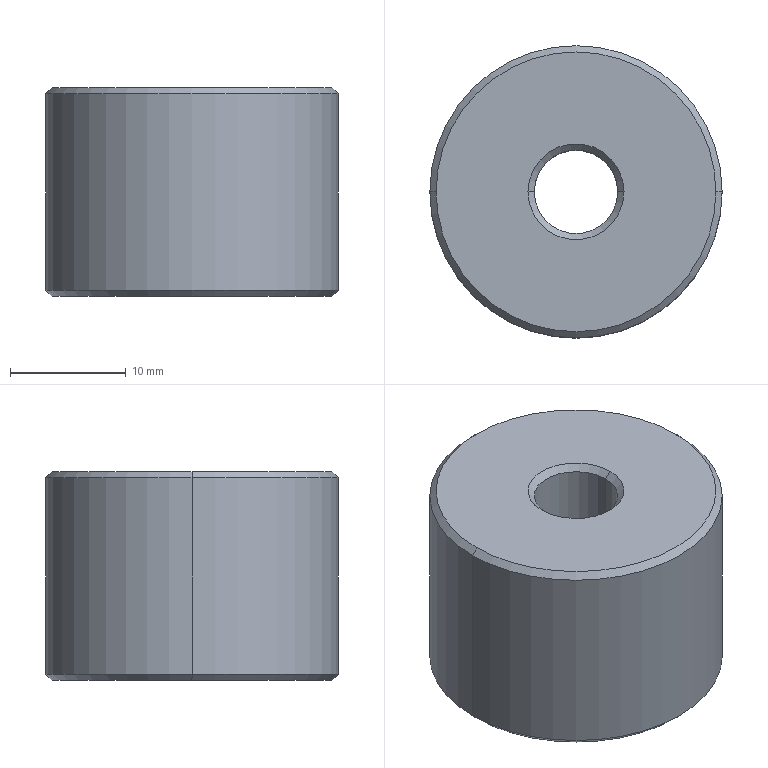Part | SolidWorks | features Chamfer 1, Extrusion 1 | 1 solid | 14 faces | box 25.2 x 25.2 x 18 mm | volume 8215 mm3 | cone 8 | cylinder 4 | plane 2 | commonest cylinder face diameters 7.2 x2 25.2 x2
STEP:
#1=CARTESIAN_POINT('',(12.06,0.,18.));
#2=VERTEX_POINT('',#1);
#3=CARTESIAN_POINT('',(-12.06,0.,18.));
#4=VERTEX_POINT('',#3);
#5=CARTESIAN_POINT('',(0.,0.,18.));
#6=DIRECTION('',(0.,0.,1.));
#7=DIRECTION('',(1.,0.,0.));
#8=AXIS2_PLACEMENT_3D('',#5,#6,#7);
#9=CIRCLE('',#8,12.06);
#10=EDGE_CURVE('',#2,#4,#9,.T.);
#11=ORIENTED_EDGE('',*,*,#10,.F.);
#12=CARTESIAN_POINT('',(12.6,0.,17.46));
#13=VERTEX_POINT('',#12);
#14=CARTESIAN_POINT('',(12.06,0.,18.));
#15=DIRECTION('',(0.7071,0.,-0.7071));
#16=VECTOR('',#15,1000.);
#17=LINE('',#14,#16);
#18=EDGE_CURVE('',#2,#13,#17,.T.);
#19=ORIENTED_EDGE('',*,*,#18,.T.);
#20=CARTESIAN_POINT('',(-12.6,0.,17.46));
#21=VERTEX_POINT('',#20);
#22=CARTESIAN_POINT('',(0.,0.,17.46));
#23=DIRECTION('',(0.,0.,-1.));
#24=DIRECTION('',(1.,0.,0.));
#25=AXIS2_PLACEMENT_3D('',#22,#23,#24);
#26=CIRCLE('',#25,12.6);
#27=EDGE_CURVE('',#21,#13,#26,.T.);
#28=ORIENTED_EDGE('',*,*,#27,.F.);
#29=CARTESIAN_POINT('',(-12.06,0.,18.));
#30=DIRECTION('',(-0.7071,0.,-0.7071));
#31=VECTOR('',#30,1000.);
#32=LINE('',#29,#31);
#33=EDGE_CURVE('',#4,#21,#32,.T.);
#34=ORIENTED_EDGE('',*,*,#33,.F.);
#35=EDGE_LOOP('',(#11,#19,#28,#34));
#36=FACE_OUTER_BOUND('',#35,.T.);
#37=CARTESIAN_POINT('',(0.,0.,18.));
#38=DIRECTION('',(0.,0.,-1.));
#39=DIRECTION('',(-1.,0.,0.));
#40=AXIS2_PLACEMENT_3D('',#37,#38,#39);
#41=CONICAL_SURFACE('',#40,12.06,0.7854);
#42=ADVANCED_FACE('',(#36),#41,.T.);
#43=CARTESIAN_POINT('',(-12.06,0.,0.));
#44=VERTEX_POINT('',#43);
#45=CARTESIAN_POINT('',(12.06,0.,0.));
#46=VERTEX_POINT('',#45);
#47=CARTESIAN_POINT('',(0.,0.,0.));
#48=DIRECTION('',(0.,0.,-1.));
#49=DIRECTION('',(1.,0.,0.));
#50=AXIS2_PLACEMENT_3D('',#47,#48,#49);
#51=CIRCLE('',#50,12.06);
#52=EDGE_CURVE('',#44,#46,#51,.T.);
#53=ORIENTED_EDGE('',*,*,#52,.F.);
#54=CARTESIAN_POINT('',(-12.6,0.,0.54));
#55=VERTEX_POINT('',#54);
#56=CARTESIAN_POINT('',(-12.6,0.,0.54));
#57=DIRECTION('',(-0.7071,0.,0.7071));
#58=VECTOR('',#57,1000.);
#59=LINE('',#56,#58);
#60=EDGE_CURVE('',#44,#55,#59,.T.);
#61=ORIENTED_EDGE('',*,*,#60,.T.);
#62=CARTESIAN_POINT('',(12.6,0.,0.54));
#63=VERTEX_POINT('',#62);
#64=CARTESIAN_POINT('',(0.,0.,0.54));
#65=DIRECTION('',(0.,0.,1.));
#66=DIRECTION('',(1.,0.,0.));
#67=AXIS2_PLACEMENT_3D('',#64,#65,#66);
#68=CIRCLE('',#67,12.6);
#69=EDGE_CURVE('',#63,#55,#68,.T.);
#70=ORIENTED_EDGE('',*,*,#69,.F.);
#71=CARTESIAN_POINT('',(12.6,0.,0.54));
#72=DIRECTION('',(0.7071,0.,0.7071));
#73=VECTOR('',#72,1000.);
#74=LINE('',#71,#73);
#75=EDGE_CURVE('',#46,#63,#74,.T.);
#76=ORIENTED_EDGE('',*,*,#75,.F.);
#77=EDGE_LOOP('',(#53,#61,#70,#76));
#78=FACE_OUTER_BOUND('',#77,.T.);
#79=CARTESIAN_POINT('',(0.,0.,0.54));
#80=DIRECTION('',(0.,0.,1.));
#81=DIRECTION('',(1.,0.,0.));
#82=AXIS2_PLACEMENT_3D('',#79,#80,#81);
#83=CONICAL_SURFACE('',#82,12.6,0.7854);
#84=ADVANCED_FACE('',(#78),#83,.T.);
#85=CARTESIAN_POINT('',(3.6,0.,0.54));
#86=VERTEX_POINT('',#85);
#87=CARTESIAN_POINT('',(-3.6,0.,0.54));
#88=VERTEX_POINT('',#87);
#89=CARTESIAN_POINT('',(0.,0.,0.54));
#90=DIRECTION('',(0.,0.,-1.));
#91=DIRECTION('',(1.,0.,0.));
#92=AXIS2_PLACEMENT_3D('',#89,#90,#91);
#93=CIRCLE('',#92,3.6);
#94=EDGE_CURVE('',#86,#88,#93,.T.);
#95=ORIENTED_EDGE('',*,*,#94,.F.);
#96=CARTESIAN_POINT('',(4.14,0.,0.));
#97=VERTEX_POINT('',#96);
#98=CARTESIAN_POINT('',(4.14,0.,0.));
#99=DIRECTION('',(0.7071,0.,-0.7071));
#100=VECTOR('',#99,1000.);
#101=LINE('',#98,#100);
#102=EDGE_CURVE('',#86,#97,#101,.T.);
#103=ORIENTED_EDGE('',*,*,#102,.T.);
#104=CARTESIAN_POINT('',(-4.14,0.,0.));
#105=VERTEX_POINT('',#104);
#106=CARTESIAN_POINT('',(0.,0.,0.));
#107=DIRECTION('',(0.,0.,1.));
#108=DIRECTION('',(1.,0.,0.));
#109=AXIS2_PLACEMENT_3D('',#106,#107,#108);
#110=CIRCLE('',#109,4.14);
#111=EDGE_CURVE('',#105,#97,#110,.T.);
#112=ORIENTED_EDGE('',*,*,#111,.F.);
#113=CARTESIAN_POINT('',(-4.14,0.,0.));
#114=DIRECTION('',(-0.7071,0.,-0.7071));
#115=VECTOR('',#114,1000.);
#116=LINE('',#113,#115);
#117=EDGE_CURVE('',#88,#105,#116,.T.);
#118=ORIENTED_EDGE('',*,*,#117,.F.);
#119=EDGE_LOOP('',(#95,#103,#112,#118));
#120=FACE_OUTER_BOUND('',#119,.T.);
#121=CARTESIAN_POINT('',(0.,0.,0.));
#122=DIRECTION('',(0.,0.,-1.));
#123=DIRECTION('',(-1.,0.,0.));
#124=AXIS2_PLACEMENT_3D('',#121,#122,#123);
#125=CONICAL_SURFACE('',#124,4.14,0.7854);
#126=ADVANCED_FACE('',(#120),#125,.F.);
#127=CARTESIAN_POINT('',(-3.6,0.,17.46));
#128=VERTEX_POINT('',#127);
#129=CARTESIAN_POINT('',(3.6,0.,17.46));
#130=VERTEX_POINT('',#129);
#131=CARTESIAN_POINT('',(0.,0.,17.46));
#132=DIRECTION('',(0.,0.,1.));
#133=DIRECTION('',(1.,0.,0.));
#134=AXIS2_PLACEMENT_3D('',#131,#132,#133);
#135=CIRCLE('',#134,3.6);
#136=EDGE_CURVE('',#128,#130,#135,.T.);
#137=ORIENTED_EDGE('',*,*,#136,.F.);
#138=CARTESIAN_POINT('',(-4.14,0.,18.));
#139=VERTEX_POINT('',#138);
#140=CARTESIAN_POINT('',(-3.6,0.,17.46));
#141=DIRECTION('',(-0.7071,0.,0.7071));
#142=VECTOR('',#141,1000.);
#143=LINE('',#140,#142);
#144=EDGE_CURVE('',#128,#139,#143,.T.);
#145=ORIENTED_EDGE('',*,*,#144,.T.);
#146=CARTESIAN_POINT('',(4.14,0.,18.));
#147=VERTEX_POINT('',#146);
#148=CARTESIAN_POINT('',(0.,0.,18.));
#149=DIRECTION('',(0.,0.,-1.));
#150=DIRECTION('',(1.,0.,0.));
#151=AXIS2_PLACEMENT_3D('',#148,#149,#150);
#152=CIRCLE('',#151,4.14);
#153=EDGE_CURVE('',#147,#139,#152,.T.);
#154=ORIENTED_EDGE('',*,*,#153,.F.);
#155=CARTESIAN_POINT('',(3.6,0.,17.46));
#156=DIRECTION('',(0.7071,0.,0.7071));
#157=VECTOR('',#156,1000.);
#158=LINE('',#155,#157);
#159=EDGE_CURVE('',#130,#147,#158,.T.);
#160=ORIENTED_EDGE('',*,*,#159,.F.);
#161=EDGE_LOOP('',(#137,#145,#154,#160));
#162=FACE_OUTER_BOUND('',#161,.T.);
#163=CARTESIAN_POINT('',(0.,0.,17.46));
#164=DIRECTION('',(0.,0.,1.));
#165=DIRECTION('',(1.,0.,0.));
#166=AXIS2_PLACEMENT_3D('',#163,#164,#165);
#167=CONICAL_SURFACE('',#166,3.6,0.7854);
#168=ADVANCED_FACE('',(#162),#167,.F.);
#169=ORIENTED_EDGE('',*,*,#136,.T.);
#170=CARTESIAN_POINT('',(3.6,0.,18.));
#171=DIRECTION('',(0.,0.,-1.));
#172=VECTOR('',#171,1000.);
#173=LINE('',#170,#172);
#174=EDGE_CURVE('',#130,#86,#173,.T.);
#175=ORIENTED_EDGE('',*,*,#174,.T.);
#176=ORIENTED_EDGE('',*,*,#94,.T.);
#177=CARTESIAN_POINT('',(-3.6,0.,18.));
#178=DIRECTION('',(0.,0.,-1.));
#179=VECTOR('',#178,1000.);
#180=LINE('',#177,#179);
#181=EDGE_CURVE('',#128,#88,#180,.T.);
#182=ORIENTED_EDGE('',*,*,#181,.F.);
#183=EDGE_LOOP('',(#169,#175,#176,#182));
#184=FACE_OUTER_BOUND('',#183,.T.);
#185=CARTESIAN_POINT('',(0.,0.,18.));
#186=DIRECTION('',(0.,0.,-1.));
#187=DIRECTION('',(-1.,0.,0.));
#188=AXIS2_PLACEMENT_3D('',#185,#186,#187);
#189=CYLINDRICAL_SURFACE('',#188,3.6);
#190=ADVANCED_FACE('',(#184),#189,.F.);
#191=ORIENTED_EDGE('',*,*,#27,.T.);
#192=CARTESIAN_POINT('',(12.6,0.,18.));
#193=DIRECTION('',(0.,0.,-1.));
#194=VECTOR('',#193,1000.);
#195=LINE('',#192,#194);
#196=EDGE_CURVE('',#13,#63,#195,.T.);
#197=ORIENTED_EDGE('',*,*,#196,.T.);
#198=ORIENTED_EDGE('',*,*,#69,.T.);
#199=CARTESIAN_POINT('',(-12.6,0.,18.));
#200=DIRECTION('',(0.,0.,-1.));
#201=VECTOR('',#200,1000.);
#202=LINE('',#199,#201);
#203=EDGE_CURVE('',#21,#55,#202,.T.);
#204=ORIENTED_EDGE('',*,*,#203,.F.);
#205=EDGE_LOOP('',(#191,#197,#198,#204));
#206=FACE_OUTER_BOUND('',#205,.T.);
#207=CARTESIAN_POINT('',(0.,0.,18.));
#208=DIRECTION('',(0.,0.,-1.));
#209=DIRECTION('',(-1.,0.,0.));
#210=AXIS2_PLACEMENT_3D('',#207,#208,#209);
#211=CYLINDRICAL_SURFACE('',#210,12.6);
#212=ADVANCED_FACE('',(#206),#211,.T.);
#213=ORIENTED_EDGE('',*,*,#153,.T.);
#214=CARTESIAN_POINT('',(0.,0.,18.));
#215=DIRECTION('',(0.,0.,-1.));
#216=DIRECTION('',(1.,0.,0.));
#217=AXIS2_PLACEMENT_3D('',#214,#215,#216);
#218=CIRCLE('',#217,4.14);
#219=EDGE_CURVE('',#139,#147,#218,.T.);
#220=ORIENTED_EDGE('',*,*,#219,.T.);
#221=EDGE_LOOP('',(#213,#220));
#222=FACE_BOUND('',#221,.T.);
#223=CARTESIAN_POINT('',(0.,0.,18.));
#224=DIRECTION('',(0.,0.,1.));
#225=DIRECTION('',(1.,0.,0.));
#226=AXIS2_PLACEMENT_3D('',#223,#224,#225);
#227=CIRCLE('',#226,12.06);
#228=EDGE_CURVE('',#4,#2,#227,.T.);
#229=ORIENTED_EDGE('',*,*,#228,.T.);
#230=ORIENTED_EDGE('',*,*,#10,.T.);
#231=EDGE_LOOP('',(#229,#230));
#232=FACE_OUTER_BOUND('',#231,.T.);
#233=CARTESIAN_POINT('',(0.,0.,18.));
#234=DIRECTION('',(0.,0.,1.));
#235=DIRECTION('',(1.,0.,0.));
#236=AXIS2_PLACEMENT_3D('',#233,#234,#235);
#237=PLANE('',#236);
#238=ADVANCED_FACE('',(#222,#232),#237,.T.);
#239=ORIENTED_EDGE('',*,*,#111,.T.);
#240=CARTESIAN_POINT('',(0.,0.,0.));
#241=DIRECTION('',(0.,0.,1.));
#242=DIRECTION('',(1.,0.,0.));
#243=AXIS2_PLACEMENT_3D('',#240,#241,#242);
#244=CIRCLE('',#243,4.14);
#245=EDGE_CURVE('',#97,#105,#244,.T.);
#246=ORIENTED_EDGE('',*,*,#245,.T.);
#247=EDGE_LOOP('',(#239,#246));
#248=FACE_BOUND('',#247,.T.);
#249=CARTESIAN_POINT('',(0.,0.,0.));
#250=DIRECTION('',(0.,0.,-1.));
#251=DIRECTION('',(1.,0.,0.));
#252=AXIS2_PLACEMENT_3D('',#249,#250,#251);
#253=CIRCLE('',#252,12.06);
#254=EDGE_CURVE('',#46,#44,#253,.T.);
#255=ORIENTED_EDGE('',*,*,#254,.T.);
#256=ORIENTED_EDGE('',*,*,#52,.T.);
#257=EDGE_LOOP('',(#255,#256));
#258=FACE_OUTER_BOUND('',#257,.T.);
#259=CARTESIAN_POINT('',(0.,0.,0.));
#260=DIRECTION('',(0.,0.,1.));
#261=DIRECTION('',(1.,0.,0.));
#262=AXIS2_PLACEMENT_3D('',#259,#260,#261);
#263=PLANE('',#262);
#264=ADVANCED_FACE('',(#248,#258),#263,.F.);
#265=ORIENTED_EDGE('',*,*,#196,.F.);
#266=CARTESIAN_POINT('',(0.,0.,17.46));
#267=DIRECTION('',(0.,0.,-1.));
#268=DIRECTION('',(1.,0.,0.));
#269=AXIS2_PLACEMENT_3D('',#266,#267,#268);
#270=CIRCLE('',#269,12.6);
#271=EDGE_CURVE('',#13,#21,#270,.T.);
#272=ORIENTED_EDGE('',*,*,#271,.T.);
#273=ORIENTED_EDGE('',*,*,#203,.T.);
#274=CARTESIAN_POINT('',(0.,0.,0.54));
#275=DIRECTION('',(0.,0.,1.));
#276=DIRECTION('',(1.,0.,0.));
#277=AXIS2_PLACEMENT_3D('',#274,#275,#276);
#278=CIRCLE('',#277,12.6);
#279=EDGE_CURVE('',#55,#63,#278,.T.);
#280=ORIENTED_EDGE('',*,*,#279,.T.);
#281=EDGE_LOOP('',(#265,#272,#273,#280));
#282=FACE_OUTER_BOUND('',#281,.T.);
#283=CARTESIAN_POINT('',(0.,0.,18.));
#284=DIRECTION('',(0.,0.,-1.));
#285=DIRECTION('',(-1.,0.,0.));
#286=AXIS2_PLACEMENT_3D('',#283,#284,#285);
#287=CYLINDRICAL_SURFACE('',#286,12.6);
#288=ADVANCED_FACE('',(#282),#287,.T.);
#289=ORIENTED_EDGE('',*,*,#174,.F.);
#290=CARTESIAN_POINT('',(0.,0.,17.46));
#291=DIRECTION('',(0.,0.,1.));
#292=DIRECTION('',(1.,0.,0.));
#293=AXIS2_PLACEMENT_3D('',#290,#291,#292);
#294=CIRCLE('',#293,3.6);
#295=EDGE_CURVE('',#130,#128,#294,.T.);
#296=ORIENTED_EDGE('',*,*,#295,.T.);
#297=ORIENTED_EDGE('',*,*,#181,.T.);
#298=CARTESIAN_POINT('',(0.,0.,0.54));
#299=DIRECTION('',(0.,0.,-1.));
#300=DIRECTION('',(1.,0.,0.));
#301=AXIS2_PLACEMENT_3D('',#298,#299,#300);
#302=CIRCLE('',#301,3.6);
#303=EDGE_CURVE('',#88,#86,#302,.T.);
#304=ORIENTED_EDGE('',*,*,#303,.T.);
#305=EDGE_LOOP('',(#289,#296,#297,#304));
#306=FACE_OUTER_BOUND('',#305,.T.);
#307=CARTESIAN_POINT('',(0.,0.,18.));
#308=DIRECTION('',(0.,0.,-1.));
#309=DIRECTION('',(-1.,0.,0.));
#310=AXIS2_PLACEMENT_3D('',#307,#308,#309);
#311=CYLINDRICAL_SURFACE('',#310,3.6);
#312=ADVANCED_FACE('',(#306),#311,.F.);
#313=ORIENTED_EDGE('',*,*,#144,.F.);
#314=ORIENTED_EDGE('',*,*,#295,.F.);
#315=ORIENTED_EDGE('',*,*,#159,.T.);
#316=ORIENTED_EDGE('',*,*,#219,.F.);
#317=EDGE_LOOP('',(#313,#314,#315,#316));
#318=FACE_OUTER_BOUND('',#317,.T.);
#319=CARTESIAN_POINT('',(0.,0.,17.46));
#320=DIRECTION('',(0.,0.,1.));
#321=DIRECTION('',(1.,0.,0.));
#322=AXIS2_PLACEMENT_3D('',#319,#320,#321);
#323=CONICAL_SURFACE('',#322,3.6,0.7854);
#324=ADVANCED_FACE('',(#318),#323,.F.);
#325=ORIENTED_EDGE('',*,*,#102,.F.);
#326=ORIENTED_EDGE('',*,*,#303,.F.);
#327=ORIENTED_EDGE('',*,*,#117,.T.);
#328=ORIENTED_EDGE('',*,*,#245,.F.);
#329=EDGE_LOOP('',(#325,#326,#327,#328));
#330=FACE_OUTER_BOUND('',#329,.T.);
#331=CARTESIAN_POINT('',(0.,0.,0.));
#332=DIRECTION('',(0.,0.,-1.));
#333=DIRECTION('',(-1.,0.,0.));
#334=AXIS2_PLACEMENT_3D('',#331,#332,#333);
#335=CONICAL_SURFACE('',#334,4.14,0.7854);
#336=ADVANCED_FACE('',(#330),#335,.F.);
#337=ORIENTED_EDGE('',*,*,#60,.F.);
#338=ORIENTED_EDGE('',*,*,#254,.F.);
#339=ORIENTED_EDGE('',*,*,#75,.T.);
#340=ORIENTED_EDGE('',*,*,#279,.F.);
#341=EDGE_LOOP('',(#337,#338,#339,#340));
#342=FACE_OUTER_BOUND('',#341,.T.);
#343=CARTESIAN_POINT('',(0.,0.,0.54));
#344=DIRECTION('',(0.,0.,1.));
#345=DIRECTION('',(1.,0.,0.));
#346=AXIS2_PLACEMENT_3D('',#343,#344,#345);
#347=CONICAL_SURFACE('',#346,12.6,0.7854);
#348=ADVANCED_FACE('',(#342),#347,.T.);
#349=ORIENTED_EDGE('',*,*,#18,.F.);
#350=ORIENTED_EDGE('',*,*,#228,.F.);
#351=ORIENTED_EDGE('',*,*,#33,.T.);
#352=ORIENTED_EDGE('',*,*,#271,.F.);
#353=EDGE_LOOP('',(#349,#350,#351,#352));
#354=FACE_OUTER_BOUND('',#353,.T.);
#355=CARTESIAN_POINT('',(0.,0.,18.));
#356=DIRECTION('',(0.,0.,-1.));
#357=DIRECTION('',(-1.,0.,0.));
#358=AXIS2_PLACEMENT_3D('',#355,#356,#357);
#359=CONICAL_SURFACE('',#358,12.06,0.7854);
#360=ADVANCED_FACE('',(#354),#359,.T.);
#361=CLOSED_SHELL('',(#42,#84,#126,#168,#190,#212,#238,#264,#288,#312,#324,#336,#348,#360));
#362=MANIFOLD_SOLID_BREP('',#361);
#363=CARTESIAN_POINT('',(0.,0.,0.));
#364=DIRECTION('',(0.,0.,1.));
#365=DIRECTION('',(1.,0.,0.));
#366=AXIS2_PLACEMENT_3D('',#363,#364,#365);
#367=(LENGTH_UNIT()NAMED_UNIT(*)SI_UNIT(.MILLI.,.METRE.));
#368=UNCERTAINTY_MEASURE_WITH_UNIT(LENGTH_MEASURE(0.00001),#367,'','');
#369=(NAMED_UNIT(*)PLANE_ANGLE_UNIT()SI_UNIT($,.RADIAN.));
#370=(NAMED_UNIT(*)SI_UNIT($,.STERADIAN.)SOLID_ANGLE_UNIT());
#371=(GEOMETRIC_REPRESENTATION_CONTEXT(3)GLOBAL_UNCERTAINTY_ASSIGNED_CONTEXT((#368))GLOBAL_UNIT_ASSIGNED_CONTEXT((#367,#369,#370))REPRESENTATION_CONTEXT('',''));
#372=ADVANCED_BREP_SHAPE_REPRESENTATION('',(#362,#366),#371);